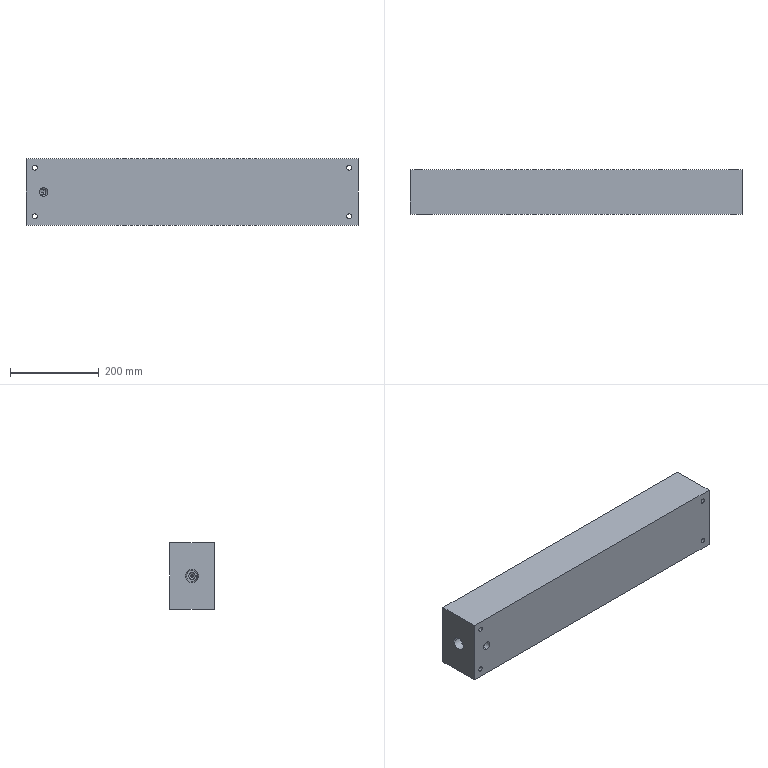Part | SolidWorks | features 3DProfileFeature 2, HoleWzd 2, Extrusion 1, ICE 1, RevCut 1 | 1 solid | 108 faces | box 750 x 100 x 150 mm | volume 11136874 mm3 | cylinder 57 | cone 39 | plane 12 | commonest cylinder face diameters 5 x32 11 x8 18 x8 6 x2 15 x2 19.5 x2